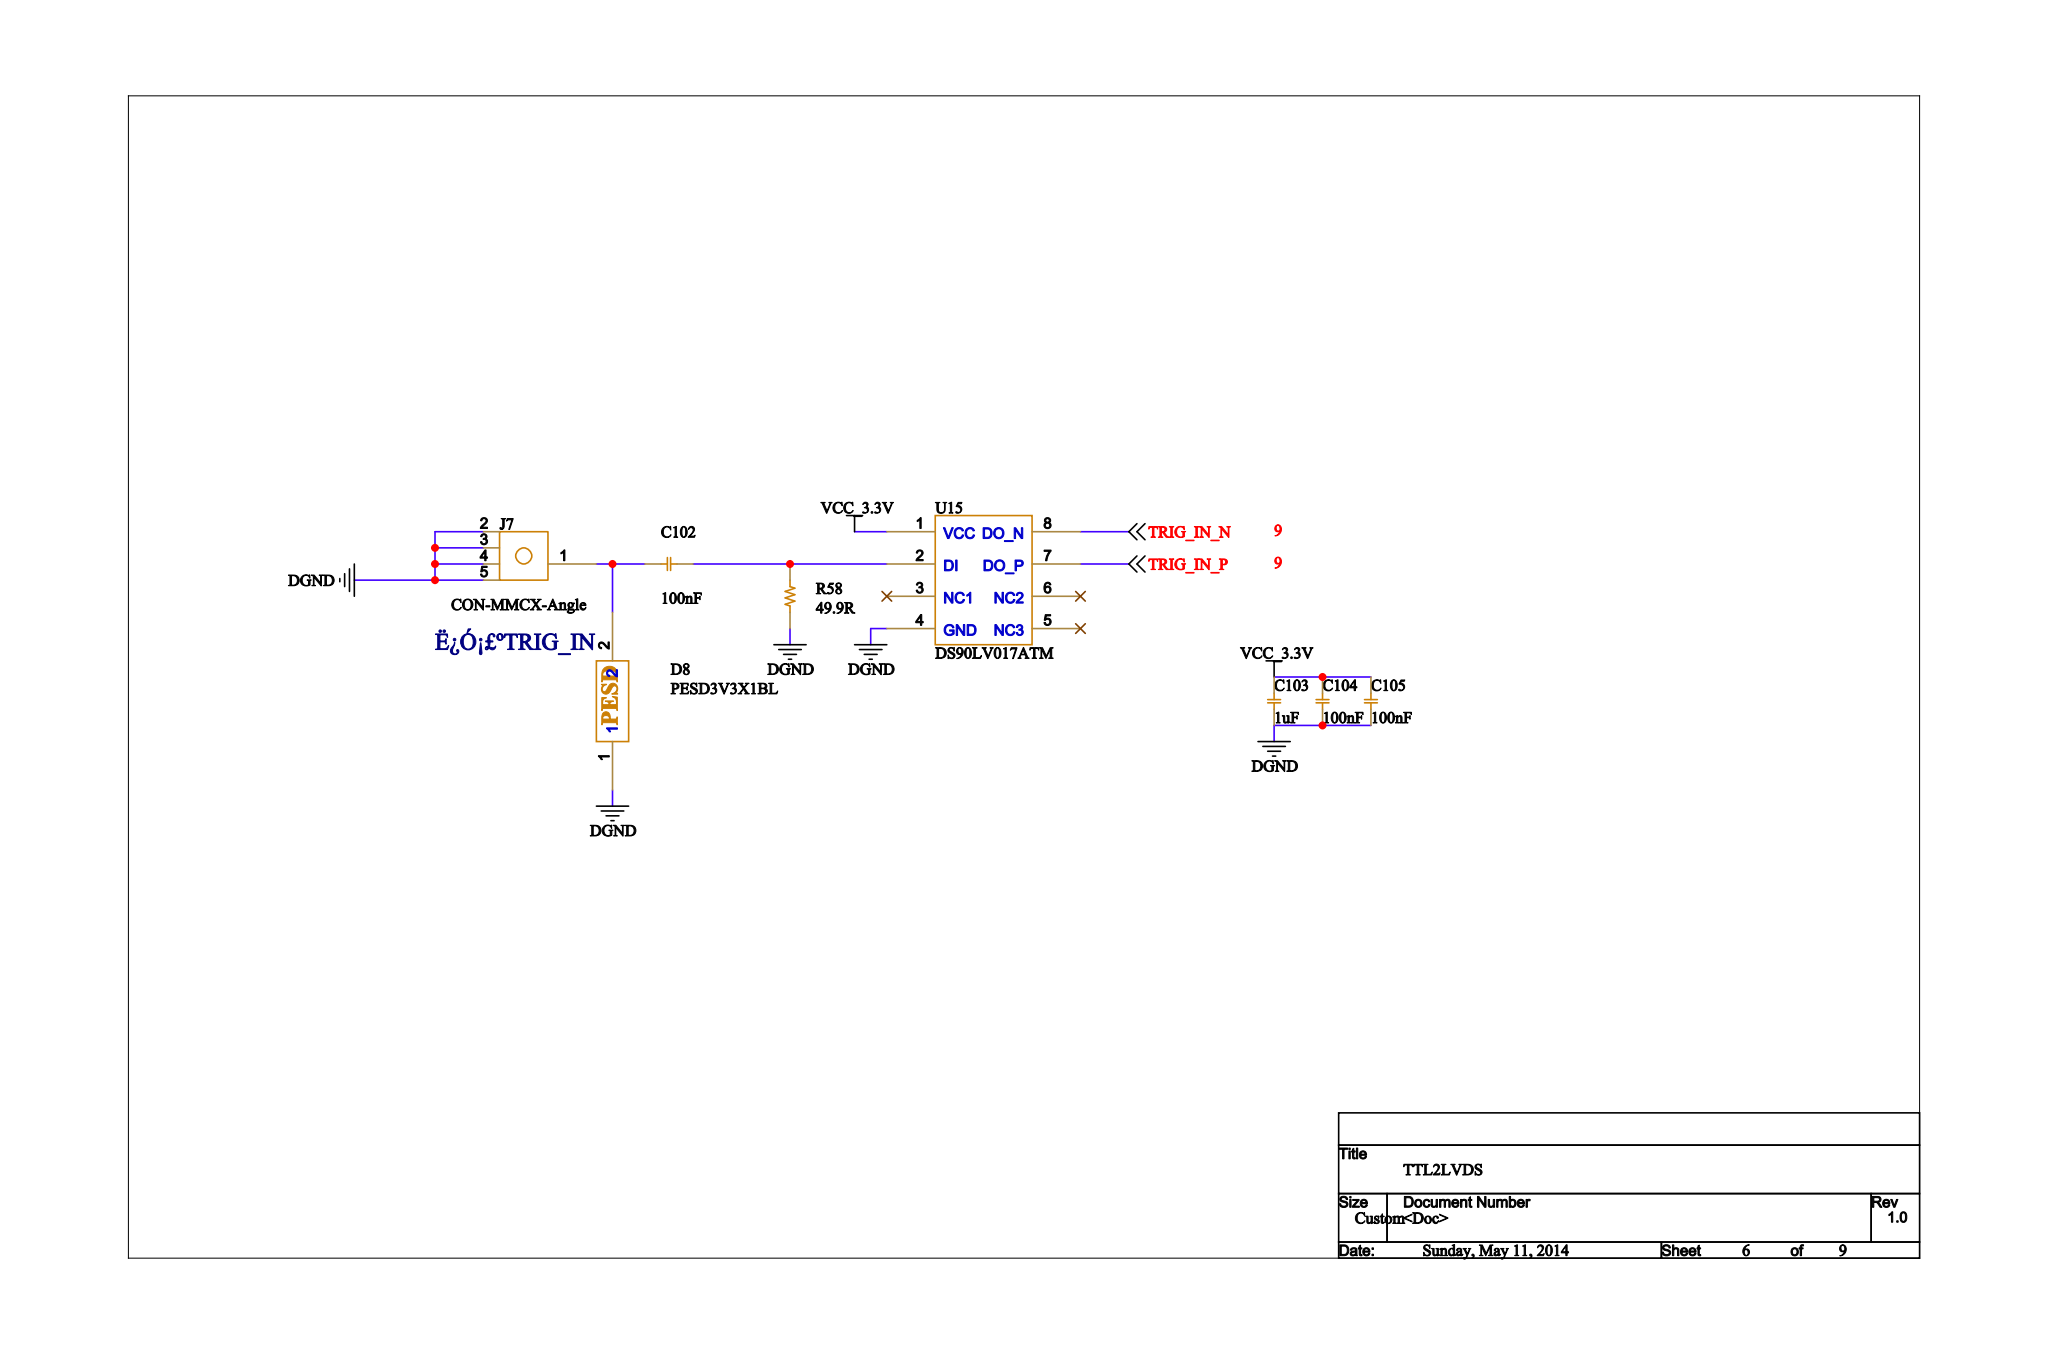Circuit board | Cadence Allegro | 233 parts | 224 nets | one sheet of the schematic
Parts on this sheet (reference | value | footprint):
C102 | 100nF | FPC-0402C
C103 | 1uF | FPC-0402C
C104 | 100nF | FPC-0402C
C105 | 100nF | FPC-0402C
D8 | PESD3V3X1BL | SOD882
J7 | CON-MMCX-Angle | SMA
R58 | 49.9R | FPC-0603R
U15 | DS90LV017ATM | FPC-SO8-150
Nets of these parts (net: part-pin ...):
DGND: C103-1 C104-1 C105-1 D8-1 J7-2 J7-3 J7-4 J7-5 R58-1 U15-4
N374382: C102-2 D8-2 J7-1
N01498: C102-1 R58-2 U15-2
VCC_3.3V: C103-2 C104-2 C105-2 U15-1
TRIG_IN_N: U15-8
TRIG_IN_P: U15-7